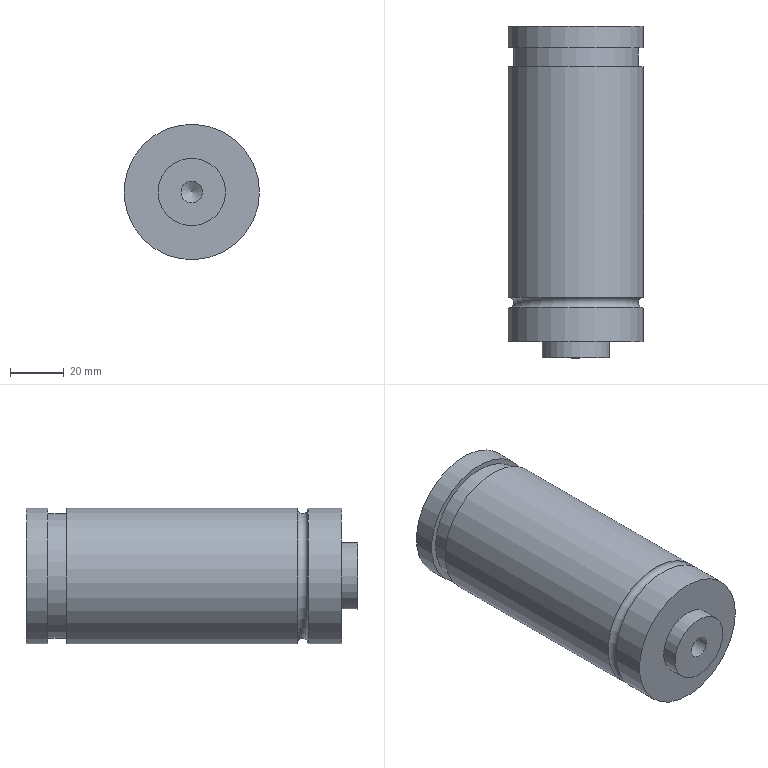Part | NX | features MAIN_BODY 2 | 1 solid | 13 faces | box 50.2 x 123 x 50.2 mm | volume 230795 mm3 | cylinder 6 | plane 5 | cone 1 | torus 1 | commonest cylinder face diameters 50.2 x3 8 x1 25 x1 46.2 x1
STEP:
#1=CARTESIAN_POINT('',(-451.9,-722.001,130.));
#2=VERTEX_POINT('',#1);
#3=CARTESIAN_POINT('',(-477.,-722.001,130.));
#4=DIRECTION('',(0.,1.,0.));
#5=DIRECTION('',(1.,0.,0.));
#6=AXIS2_PLACEMENT_3D('',#3,#4,#5);
#7=CIRCLE('',#6,25.1);
#8=EDGE_CURVE('',#2,#2,#7,.T.);
#9=ORIENTED_EDGE('',*,*,#8,.F.);
#10=EDGE_LOOP('',(#9));
#11=FACE_BOUND('',#10,.T.);
#12=CARTESIAN_POINT('',(-464.5,-722.001,130.));
#13=VERTEX_POINT('',#12);
#14=CARTESIAN_POINT('',(-477.,-722.001,130.));
#15=DIRECTION('',(0.,1.,0.));
#16=DIRECTION('',(1.,0.,0.));
#17=AXIS2_PLACEMENT_3D('',#14,#15,#16);
#18=CIRCLE('',#17,12.5);
#19=EDGE_CURVE('',#13,#13,#18,.T.);
#20=ORIENTED_EDGE('',*,*,#19,.T.);
#21=EDGE_LOOP('',(#20));
#22=FACE_BOUND('',#21,.T.);
#23=CARTESIAN_POINT('',(-477.,-722.001,130.));
#24=DIRECTION('',(0.,-1.,0.));
#25=DIRECTION('',(1.,0.,0.));
#26=AXIS2_PLACEMENT_3D('',#23,#24,#25);
#27=PLANE('',#26);
#28=ADVANCED_FACE('',(#11,#22),#27,.T.);
#29=CARTESIAN_POINT('',(-451.9,-709.501,130.));
#30=VERTEX_POINT('',#29);
#31=CARTESIAN_POINT('',(-477.,-709.501,130.));
#32=DIRECTION('',(0.,1.,0.));
#33=DIRECTION('',(1.,0.,0.));
#34=AXIS2_PLACEMENT_3D('',#31,#32,#33);
#35=CIRCLE('',#34,25.1);
#36=EDGE_CURVE('',#30,#30,#35,.T.);
#37=ORIENTED_EDGE('',*,*,#36,.F.);
#38=EDGE_LOOP('',(#37));
#39=FACE_BOUND('',#38,.T.);
#40=ORIENTED_EDGE('',*,*,#8,.T.);
#41=EDGE_LOOP('',(#40));
#42=FACE_BOUND('',#41,.T.);
#43=CARTESIAN_POINT('',(-477.,-722.001,130.));
#44=DIRECTION('',(0.,1.,0.));
#45=DIRECTION('',(-1.,0.,0.));
#46=AXIS2_PLACEMENT_3D('',#43,#44,#45);
#47=CYLINDRICAL_SURFACE('',#46,25.1);
#48=ADVANCED_FACE('',(#39,#42),#47,.T.);
#49=CARTESIAN_POINT('',(-464.5,-728.001,130.));
#50=VERTEX_POINT('',#49);
#51=CARTESIAN_POINT('',(-477.,-728.001,130.));
#52=DIRECTION('',(0.,1.,0.));
#53=DIRECTION('',(1.,0.,0.));
#54=AXIS2_PLACEMENT_3D('',#51,#52,#53);
#55=CIRCLE('',#54,12.5);
#56=EDGE_CURVE('',#50,#50,#55,.T.);
#57=ORIENTED_EDGE('',*,*,#56,.T.);
#58=EDGE_LOOP('',(#57));
#59=FACE_BOUND('',#58,.T.);
#60=ORIENTED_EDGE('',*,*,#19,.F.);
#61=EDGE_LOOP('',(#60));
#62=FACE_BOUND('',#61,.T.);
#63=CARTESIAN_POINT('',(-477.,-728.001,130.));
#64=DIRECTION('',(0.,1.,0.));
#65=DIRECTION('',(-1.,0.,0.));
#66=AXIS2_PLACEMENT_3D('',#63,#64,#65);
#67=CYLINDRICAL_SURFACE('',#66,12.5);
#68=ADVANCED_FACE('',(#59,#62),#67,.T.);
#69=CARTESIAN_POINT('',(-481.,-728.001,130.));
#70=VERTEX_POINT('',#69);
#71=CARTESIAN_POINT('',(-477.,-728.001,130.));
#72=DIRECTION('',(0.,-1.,0.));
#73=DIRECTION('',(-1.,0.,0.));
#74=AXIS2_PLACEMENT_3D('',#71,#72,#73);
#75=CIRCLE('',#74,4.);
#76=EDGE_CURVE('',#70,#70,#75,.T.);
#77=ORIENTED_EDGE('',*,*,#76,.F.);
#78=EDGE_LOOP('',(#77));
#79=FACE_BOUND('',#78,.T.);
#80=ORIENTED_EDGE('',*,*,#56,.F.);
#81=EDGE_LOOP('',(#80));
#82=FACE_BOUND('',#81,.T.);
#83=CARTESIAN_POINT('',(-477.,-728.001,130.));
#84=DIRECTION('',(0.,-1.,0.));
#85=DIRECTION('',(1.,0.,0.));
#86=AXIS2_PLACEMENT_3D('',#83,#84,#85);
#87=PLANE('',#86);
#88=ADVANCED_FACE('',(#79,#82),#87,.T.);
#89=CARTESIAN_POINT('',(-481.,-716.001,130.));
#90=VERTEX_POINT('',#89);
#91=CARTESIAN_POINT('',(-477.,-716.001,130.));
#92=DIRECTION('',(0.,-1.,0.));
#93=DIRECTION('',(-1.,0.,0.));
#94=AXIS2_PLACEMENT_3D('',#91,#92,#93);
#95=CIRCLE('',#94,4.);
#96=EDGE_CURVE('',#90,#90,#95,.T.);
#97=ORIENTED_EDGE('',*,*,#96,.T.);
#98=EDGE_LOOP('',(#97));
#99=FACE_BOUND('',#98,.T.);
#100=CARTESIAN_POINT('',(-477.,-713.597,130.));
#101=VERTEX_POINT('',#100);
#102=VERTEX_LOOP('',#101);
#103=FACE_BOUND('',#102,.T.);
#104=CARTESIAN_POINT('',(-477.,-716.001,130.));
#105=DIRECTION('',(0.,-1.,0.));
#106=DIRECTION('',(1.,0.,0.));
#107=AXIS2_PLACEMENT_3D('',#104,#105,#106);
#108=CONICAL_SURFACE('',#107,4.,1.03);
#109=ADVANCED_FACE('',(#99,#103),#108,.F.);
#110=ORIENTED_EDGE('',*,*,#96,.F.);
#111=EDGE_LOOP('',(#110));
#112=FACE_BOUND('',#111,.T.);
#113=ORIENTED_EDGE('',*,*,#76,.T.);
#114=EDGE_LOOP('',(#113));
#115=FACE_BOUND('',#114,.T.);
#116=CARTESIAN_POINT('',(-477.,-728.001,130.));
#117=DIRECTION('',(0.,1.,0.));
#118=DIRECTION('',(-1.,0.,0.));
#119=AXIS2_PLACEMENT_3D('',#116,#117,#118);
#120=CYLINDRICAL_SURFACE('',#119,4.);
#121=ADVANCED_FACE('',(#112,#115),#120,.F.);
#122=ORIENTED_EDGE('',*,*,#36,.T.);
#123=EDGE_LOOP('',(#122));
#124=FACE_BOUND('',#123,.T.);
#125=CARTESIAN_POINT('',(-451.9,-705.501,130.));
#126=VERTEX_POINT('',#125);
#127=CARTESIAN_POINT('',(-477.,-705.501,130.));
#128=DIRECTION('',(0.,1.,0.));
#129=DIRECTION('',(1.,0.,0.));
#130=AXIS2_PLACEMENT_3D('',#127,#128,#129);
#131=CIRCLE('',#130,25.1);
#132=EDGE_CURVE('',#126,#126,#131,.T.);
#133=ORIENTED_EDGE('',*,*,#132,.F.);
#134=EDGE_LOOP('',(#133));
#135=FACE_BOUND('',#134,.T.);
#136=CARTESIAN_POINT('',(-477.,-707.501,130.));
#137=DIRECTION('',(0.,-1.,0.));
#138=DIRECTION('',(1.,0.,0.));
#139=AXIS2_PLACEMENT_3D('',#136,#137,#138);
#140=TOROIDAL_SURFACE('',#139,25.1,2.);
#141=ADVANCED_FACE('',(#124,#135),#140,.F.);
#142=CARTESIAN_POINT('',(-451.9,-620.001,130.));
#143=VERTEX_POINT('',#142);
#144=CARTESIAN_POINT('',(-477.,-620.001,130.));
#145=DIRECTION('',(0.,1.,0.));
#146=DIRECTION('',(1.,0.,0.));
#147=AXIS2_PLACEMENT_3D('',#144,#145,#146);
#148=CIRCLE('',#147,25.1);
#149=EDGE_CURVE('',#143,#143,#148,.T.);
#150=ORIENTED_EDGE('',*,*,#149,.F.);
#151=EDGE_LOOP('',(#150));
#152=FACE_BOUND('',#151,.T.);
#153=ORIENTED_EDGE('',*,*,#132,.T.);
#154=EDGE_LOOP('',(#153));
#155=FACE_BOUND('',#154,.T.);
#156=CARTESIAN_POINT('',(-477.,-722.001,130.));
#157=DIRECTION('',(0.,1.,0.));
#158=DIRECTION('',(-1.,0.,0.));
#159=AXIS2_PLACEMENT_3D('',#156,#157,#158);
#160=CYLINDRICAL_SURFACE('',#159,25.1);
#161=ADVANCED_FACE('',(#152,#155),#160,.T.);
#162=CARTESIAN_POINT('',(-453.9,-613.001,130.));
#163=VERTEX_POINT('',#162);
#164=CARTESIAN_POINT('',(-477.,-613.001,130.));
#165=DIRECTION('',(0.,1.,0.));
#166=DIRECTION('',(1.,0.,0.));
#167=AXIS2_PLACEMENT_3D('',#164,#165,#166);
#168=CIRCLE('',#167,23.1);
#169=EDGE_CURVE('',#163,#163,#168,.T.);
#170=ORIENTED_EDGE('',*,*,#169,.T.);
#171=EDGE_LOOP('',(#170));
#172=FACE_BOUND('',#171,.T.);
#173=CARTESIAN_POINT('',(-451.9,-613.001,130.));
#174=VERTEX_POINT('',#173);
#175=CARTESIAN_POINT('',(-477.,-613.001,130.));
#176=DIRECTION('',(0.,1.,0.));
#177=DIRECTION('',(1.,0.,0.));
#178=AXIS2_PLACEMENT_3D('',#175,#176,#177);
#179=CIRCLE('',#178,25.1);
#180=EDGE_CURVE('',#174,#174,#179,.T.);
#181=ORIENTED_EDGE('',*,*,#180,.F.);
#182=EDGE_LOOP('',(#181));
#183=FACE_BOUND('',#182,.T.);
#184=CARTESIAN_POINT('',(-477.,-613.001,130.));
#185=DIRECTION('',(0.,-1.,0.));
#186=DIRECTION('',(1.,0.,0.));
#187=AXIS2_PLACEMENT_3D('',#184,#185,#186);
#188=PLANE('',#187);
#189=ADVANCED_FACE('',(#172,#183),#188,.T.);
#190=CARTESIAN_POINT('',(-453.9,-620.001,130.));
#191=VERTEX_POINT('',#190);
#192=CARTESIAN_POINT('',(-477.,-620.001,130.));
#193=DIRECTION('',(0.,1.,0.));
#194=DIRECTION('',(1.,0.,0.));
#195=AXIS2_PLACEMENT_3D('',#192,#193,#194);
#196=CIRCLE('',#195,23.1);
#197=EDGE_CURVE('',#191,#191,#196,.T.);
#198=ORIENTED_EDGE('',*,*,#197,.F.);
#199=EDGE_LOOP('',(#198));
#200=FACE_BOUND('',#199,.T.);
#201=ORIENTED_EDGE('',*,*,#149,.T.);
#202=EDGE_LOOP('',(#201));
#203=FACE_BOUND('',#202,.T.);
#204=CARTESIAN_POINT('',(-477.,-620.001,130.));
#205=DIRECTION('',(0.,-1.,0.));
#206=DIRECTION('',(1.,0.,0.));
#207=AXIS2_PLACEMENT_3D('',#204,#205,#206);
#208=PLANE('',#207);
#209=ADVANCED_FACE('',(#200,#203),#208,.F.);
#210=ORIENTED_EDGE('',*,*,#197,.T.);
#211=EDGE_LOOP('',(#210));
#212=FACE_BOUND('',#211,.T.);
#213=ORIENTED_EDGE('',*,*,#169,.F.);
#214=EDGE_LOOP('',(#213));
#215=FACE_BOUND('',#214,.T.);
#216=CARTESIAN_POINT('',(-477.,-616.501,130.));
#217=DIRECTION('',(0.,-1.,0.));
#218=DIRECTION('',(1.,0.,0.));
#219=AXIS2_PLACEMENT_3D('',#216,#217,#218);
#220=CYLINDRICAL_SURFACE('',#219,23.1);
#221=ADVANCED_FACE('',(#212,#215),#220,.T.);
#222=CARTESIAN_POINT('',(-451.9,-605.001,130.));
#223=VERTEX_POINT('',#222);
#224=CARTESIAN_POINT('',(-477.,-605.001,130.));
#225=DIRECTION('',(0.,1.,0.));
#226=DIRECTION('',(1.,0.,0.));
#227=AXIS2_PLACEMENT_3D('',#224,#225,#226);
#228=CIRCLE('',#227,25.1);
#229=EDGE_CURVE('',#223,#223,#228,.T.);
#230=ORIENTED_EDGE('',*,*,#229,.T.);
#231=EDGE_LOOP('',(#230));
#232=FACE_BOUND('',#231,.T.);
#233=CARTESIAN_POINT('',(-477.,-605.001,130.));
#234=DIRECTION('',(0.,-1.,0.));
#235=DIRECTION('',(1.,0.,0.));
#236=AXIS2_PLACEMENT_3D('',#233,#234,#235);
#237=PLANE('',#236);
#238=ADVANCED_FACE('',(#232),#237,.F.);
#239=ORIENTED_EDGE('',*,*,#229,.F.);
#240=EDGE_LOOP('',(#239));
#241=FACE_BOUND('',#240,.T.);
#242=ORIENTED_EDGE('',*,*,#180,.T.);
#243=EDGE_LOOP('',(#242));
#244=FACE_BOUND('',#243,.T.);
#245=CARTESIAN_POINT('',(-477.,-722.001,130.));
#246=DIRECTION('',(0.,1.,0.));
#247=DIRECTION('',(-1.,0.,0.));
#248=AXIS2_PLACEMENT_3D('',#245,#246,#247);
#249=CYLINDRICAL_SURFACE('',#248,25.1);
#250=ADVANCED_FACE('',(#241,#244),#249,.T.);
#251=CLOSED_SHELL('',(#28,#48,#68,#88,#109,#121,#141,#161,#189,#209,#221,#238,#250));
#252=MANIFOLD_SOLID_BREP('',#251);
#253=(LENGTH_UNIT()NAMED_UNIT(*)SI_UNIT(.MILLI.,.METRE.));
#254=UNCERTAINTY_MEASURE_WITH_UNIT(LENGTH_MEASURE(0.00001),#253,'','');
#255=(NAMED_UNIT(*)PLANE_ANGLE_UNIT()SI_UNIT($,.RADIAN.));
#256=(NAMED_UNIT(*)SI_UNIT($,.STERADIAN.)SOLID_ANGLE_UNIT());
#257=(GEOMETRIC_REPRESENTATION_CONTEXT(3)GLOBAL_UNCERTAINTY_ASSIGNED_CONTEXT((#254))GLOBAL_UNIT_ASSIGNED_CONTEXT((#253,#255,#256))REPRESENTATION_CONTEXT('',''));
#258=ADVANCED_BREP_SHAPE_REPRESENTATION('',(#252),#257);